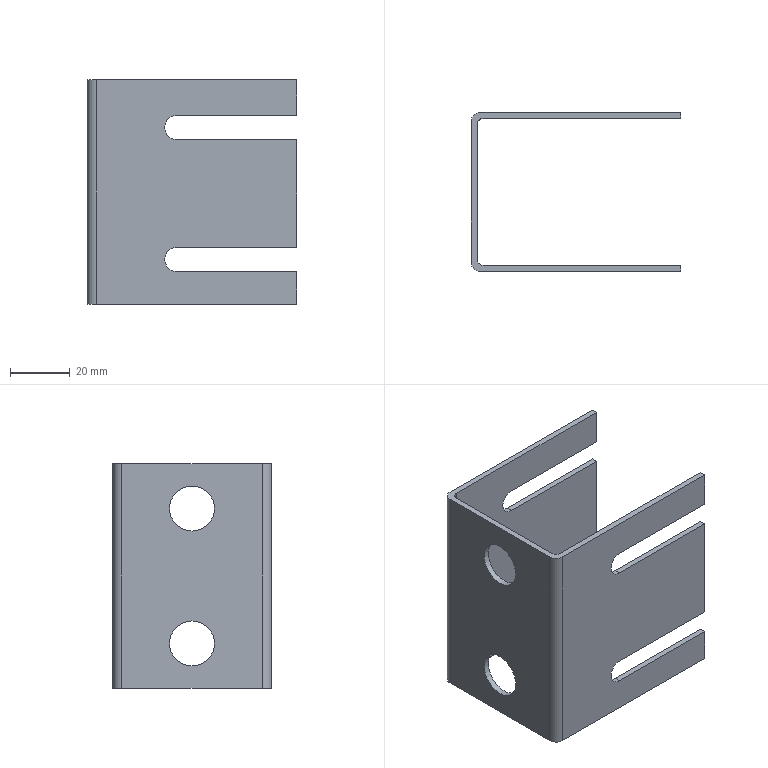Part | STEP file | Channel 30x25x3x5-50 GOST 8278-83 | 1 solid | 32 faces | box 70 x 53 x 75 mm | volume 24715 mm3 | plane 22 | cylinder 10 | commonest cylinder face diameters 8 x4 4 x2 6 x2 15 x2